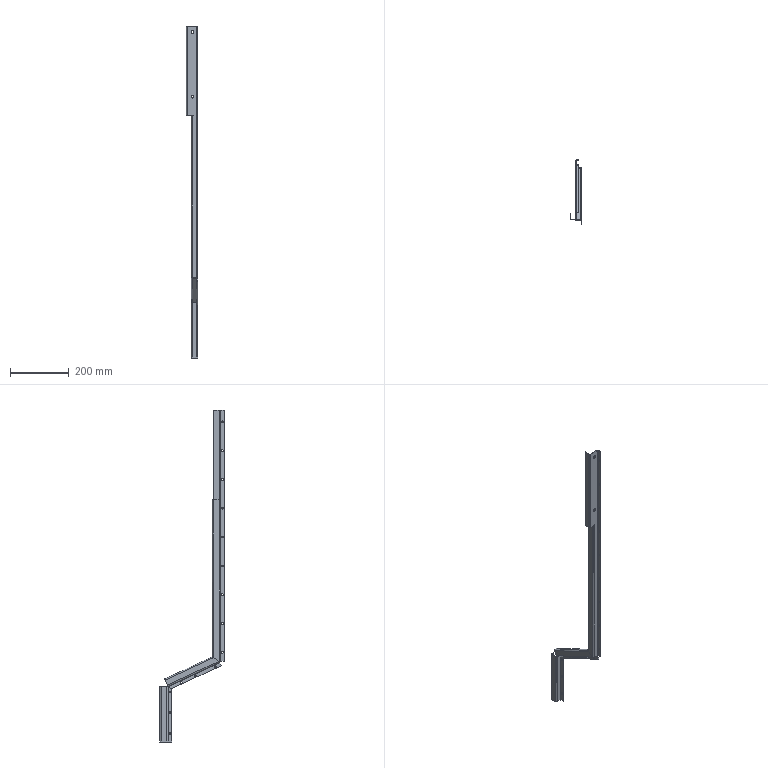Part | NX | features solid 2 | 1 solid | 128 faces | box 40 x 218 x 1127 mm | volume 161662 mm3 | plane 64 | cylinder 58 | spline 6 | commonest cylinder face diameters 6 x30 4 x12 8 x12 9.2 x4